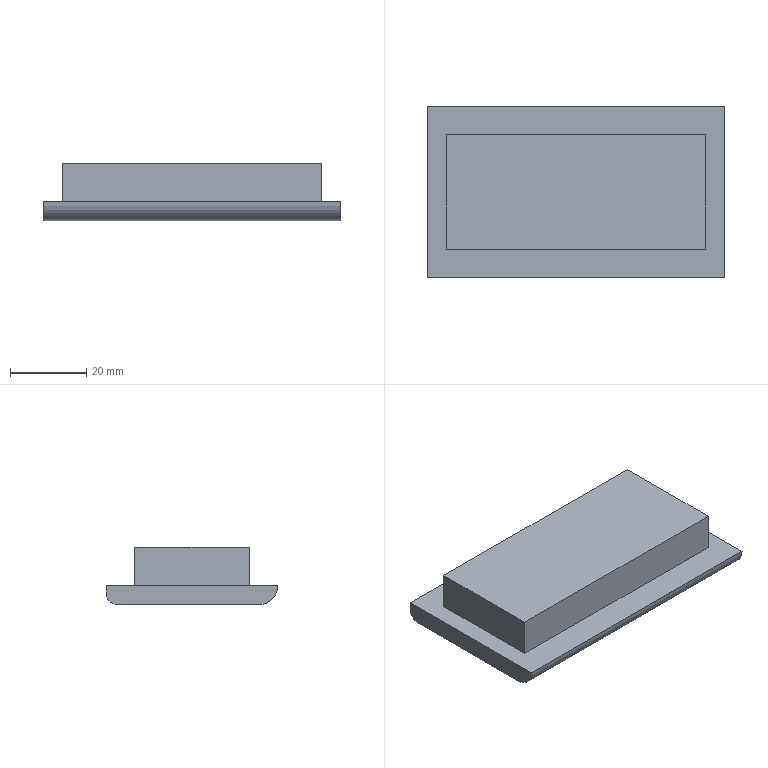Part | SolidWorks | features Fillet 3, ICE 2, Extrusion 1 | 1 solid | 18 faces | box 78 x 45 x 15 mm | volume 24133 mm3 | plane 15 | cylinder 3 | commonest cylinder face diameters 10 x2 6 x1
STEP:
#1=CARTESIAN_POINT('',(-39.,22.5,5.));
#2=VERTEX_POINT('',#1);
#3=CARTESIAN_POINT('',(-39.,-22.5,5.));
#4=VERTEX_POINT('',#3);
#5=CARTESIAN_POINT('',(-39.,-22.5,5.));
#6=DIRECTION('',(0.,-1.,0.));
#7=VECTOR('',#6,1000.);
#8=LINE('',#5,#7);
#9=EDGE_CURVE('',#2,#4,#8,.T.);
#10=ORIENTED_EDGE('',*,*,#9,.T.);
#11=CARTESIAN_POINT('',(39.,-22.5,5.));
#12=VERTEX_POINT('',#11);
#13=CARTESIAN_POINT('',(39.,-22.5,5.));
#14=DIRECTION('',(1.,0.,0.));
#15=VECTOR('',#14,1000.);
#16=LINE('',#13,#15);
#17=EDGE_CURVE('',#4,#12,#16,.T.);
#18=ORIENTED_EDGE('',*,*,#17,.T.);
#19=CARTESIAN_POINT('',(39.,22.5,5.));
#20=VERTEX_POINT('',#19);
#21=CARTESIAN_POINT('',(39.,-22.5,5.));
#22=DIRECTION('',(0.,1.,0.));
#23=VECTOR('',#22,1000.);
#24=LINE('',#21,#23);
#25=EDGE_CURVE('',#12,#20,#24,.T.);
#26=ORIENTED_EDGE('',*,*,#25,.T.);
#27=CARTESIAN_POINT('',(39.,22.5,5.));
#28=DIRECTION('',(-1.,0.,0.));
#29=VECTOR('',#28,1000.);
#30=LINE('',#27,#29);
#31=EDGE_CURVE('',#20,#2,#30,.T.);
#32=ORIENTED_EDGE('',*,*,#31,.T.);
#33=EDGE_LOOP('',(#10,#18,#26,#32));
#34=FACE_OUTER_BOUND('',#33,.T.);
#35=CARTESIAN_POINT('',(-34.,-15.,5.));
#36=VERTEX_POINT('',#35);
#37=CARTESIAN_POINT('',(34.,-15.,5.));
#38=VERTEX_POINT('',#37);
#39=CARTESIAN_POINT('',(34.,-15.,5.));
#40=DIRECTION('',(1.,0.,0.));
#41=VECTOR('',#40,1000.);
#42=LINE('',#39,#41);
#43=EDGE_CURVE('',#36,#38,#42,.T.);
#44=ORIENTED_EDGE('',*,*,#43,.F.);
#45=CARTESIAN_POINT('',(-34.,15.,5.));
#46=VERTEX_POINT('',#45);
#47=CARTESIAN_POINT('',(-34.,-15.,5.));
#48=DIRECTION('',(0.,-1.,0.));
#49=VECTOR('',#48,1000.);
#50=LINE('',#47,#49);
#51=EDGE_CURVE('',#46,#36,#50,.T.);
#52=ORIENTED_EDGE('',*,*,#51,.F.);
#53=CARTESIAN_POINT('',(34.,15.,5.));
#54=VERTEX_POINT('',#53);
#55=CARTESIAN_POINT('',(34.,15.,5.));
#56=DIRECTION('',(-1.,0.,0.));
#57=VECTOR('',#56,1000.);
#58=LINE('',#55,#57);
#59=EDGE_CURVE('',#54,#46,#58,.T.);
#60=ORIENTED_EDGE('',*,*,#59,.F.);
#61=CARTESIAN_POINT('',(34.,-15.,5.));
#62=DIRECTION('',(0.,1.,0.));
#63=VECTOR('',#62,1000.);
#64=LINE('',#61,#63);
#65=EDGE_CURVE('',#38,#54,#64,.T.);
#66=ORIENTED_EDGE('',*,*,#65,.F.);
#67=EDGE_LOOP('',(#44,#52,#60,#66));
#68=FACE_BOUND('',#67,.T.);
#69=CARTESIAN_POINT('',(-39.,22.5,5.));
#70=DIRECTION('',(0.,0.,1.));
#71=DIRECTION('',(1.,0.,0.));
#72=AXIS2_PLACEMENT_3D('',#69,#70,#71);
#73=PLANE('',#72);
#74=ADVANCED_FACE('',(#34,#68),#73,.T.);
#75=CARTESIAN_POINT('',(-39.,19.5,0.));
#76=VERTEX_POINT('',#75);
#77=CARTESIAN_POINT('',(-39.,-17.5,0.));
#78=VERTEX_POINT('',#77);
#79=CARTESIAN_POINT('',(-39.,-22.5,0.));
#80=DIRECTION('',(0.,-1.,0.));
#81=VECTOR('',#80,1000.);
#82=LINE('',#79,#81);
#83=EDGE_CURVE('',#76,#78,#82,.T.);
#84=ORIENTED_EDGE('',*,*,#83,.T.);
#85=CARTESIAN_POINT('',(-39.,-17.5,5.));
#86=DIRECTION('',(-1.,0.,0.));
#87=DIRECTION('',(0.,0.,-1.));
#88=AXIS2_PLACEMENT_3D('',#85,#86,#87);
#89=CIRCLE('',#88,5.);
#90=EDGE_CURVE('',#78,#4,#89,.T.);
#91=ORIENTED_EDGE('',*,*,#90,.T.);
#92=ORIENTED_EDGE('',*,*,#9,.F.);
#93=CARTESIAN_POINT('',(-39.,22.5,3.));
#94=VERTEX_POINT('',#93);
#95=CARTESIAN_POINT('',(-39.,22.5,5.));
#96=DIRECTION('',(0.,0.,-1.));
#97=VECTOR('',#96,1000.);
#98=LINE('',#95,#97);
#99=EDGE_CURVE('',#2,#94,#98,.T.);
#100=ORIENTED_EDGE('',*,*,#99,.T.);
#101=CARTESIAN_POINT('',(-39.,19.5,3.));
#102=DIRECTION('',(-1.,0.,0.));
#103=DIRECTION('',(0.,0.,-1.));
#104=AXIS2_PLACEMENT_3D('',#101,#102,#103);
#105=CIRCLE('',#104,3.);
#106=EDGE_CURVE('',#94,#76,#105,.T.);
#107=ORIENTED_EDGE('',*,*,#106,.T.);
#108=EDGE_LOOP('',(#84,#91,#92,#100,#107));
#109=FACE_OUTER_BOUND('',#108,.T.);
#110=CARTESIAN_POINT('',(-39.,-22.5,5.));
#111=DIRECTION('',(1.,0.,0.));
#112=DIRECTION('',(0.,0.,-1.));
#113=AXIS2_PLACEMENT_3D('',#110,#111,#112);
#114=PLANE('',#113);
#115=ADVANCED_FACE('',(#109),#114,.F.);
#116=ORIENTED_EDGE('',*,*,#25,.F.);
#117=CARTESIAN_POINT('',(39.,-17.5,0.));
#118=VERTEX_POINT('',#117);
#119=CARTESIAN_POINT('',(39.,-17.5,5.));
#120=DIRECTION('',(1.,0.,0.));
#121=DIRECTION('',(0.,0.,1.));
#122=AXIS2_PLACEMENT_3D('',#119,#120,#121);
#123=CIRCLE('',#122,5.);
#124=EDGE_CURVE('',#12,#118,#123,.T.);
#125=ORIENTED_EDGE('',*,*,#124,.T.);
#126=CARTESIAN_POINT('',(39.,19.5,0.));
#127=VERTEX_POINT('',#126);
#128=CARTESIAN_POINT('',(39.,-22.5,0.));
#129=DIRECTION('',(0.,1.,0.));
#130=VECTOR('',#129,1000.);
#131=LINE('',#128,#130);
#132=EDGE_CURVE('',#118,#127,#131,.T.);
#133=ORIENTED_EDGE('',*,*,#132,.T.);
#134=CARTESIAN_POINT('',(39.,22.5,3.));
#135=VERTEX_POINT('',#134);
#136=CARTESIAN_POINT('',(39.,19.5,3.));
#137=DIRECTION('',(1.,0.,0.));
#138=DIRECTION('',(0.,0.,1.));
#139=AXIS2_PLACEMENT_3D('',#136,#137,#138);
#140=CIRCLE('',#139,3.);
#141=EDGE_CURVE('',#127,#135,#140,.T.);
#142=ORIENTED_EDGE('',*,*,#141,.T.);
#143=CARTESIAN_POINT('',(39.,22.5,5.));
#144=DIRECTION('',(0.,0.,-1.));
#145=VECTOR('',#144,1000.);
#146=LINE('',#143,#145);
#147=EDGE_CURVE('',#20,#135,#146,.T.);
#148=ORIENTED_EDGE('',*,*,#147,.F.);
#149=EDGE_LOOP('',(#116,#125,#133,#142,#148));
#150=FACE_OUTER_BOUND('',#149,.T.);
#151=CARTESIAN_POINT('',(39.,-22.5,5.));
#152=DIRECTION('',(-1.,0.,0.));
#153=DIRECTION('',(0.,0.,1.));
#154=AXIS2_PLACEMENT_3D('',#151,#152,#153);
#155=PLANE('',#154);
#156=ADVANCED_FACE('',(#150),#155,.F.);
#157=ORIENTED_EDGE('',*,*,#147,.T.);
#158=CARTESIAN_POINT('',(39.,22.5,3.));
#159=DIRECTION('',(-1.,0.,0.));
#160=VECTOR('',#159,1000.);
#161=LINE('',#158,#160);
#162=EDGE_CURVE('',#135,#94,#161,.T.);
#163=ORIENTED_EDGE('',*,*,#162,.T.);
#164=ORIENTED_EDGE('',*,*,#99,.F.);
#165=ORIENTED_EDGE('',*,*,#31,.F.);
#166=EDGE_LOOP('',(#157,#163,#164,#165));
#167=FACE_OUTER_BOUND('',#166,.T.);
#168=CARTESIAN_POINT('',(39.,22.5,5.));
#169=DIRECTION('',(0.,-1.,0.));
#170=DIRECTION('',(1.,0.,0.));
#171=AXIS2_PLACEMENT_3D('',#168,#169,#170);
#172=PLANE('',#171);
#173=ADVANCED_FACE('',(#167),#172,.F.);
#174=CARTESIAN_POINT('',(29.243,-11.594,0.));
#175=VERTEX_POINT('',#174);
#176=CARTESIAN_POINT('',(-29.243,-11.594,0.));
#177=VERTEX_POINT('',#176);
#178=CARTESIAN_POINT('',(-29.243,-11.594,0.));
#179=DIRECTION('',(-1.,0.,0.));
#180=VECTOR('',#179,1000.);
#181=LINE('',#178,#180);
#182=EDGE_CURVE('',#175,#177,#181,.T.);
#183=ORIENTED_EDGE('',*,*,#182,.F.);
#184=CARTESIAN_POINT('',(29.243,11.594,0.));
#185=VERTEX_POINT('',#184);
#186=CARTESIAN_POINT('',(29.243,-11.594,0.));
#187=DIRECTION('',(0.,-1.,0.));
#188=VECTOR('',#187,1000.);
#189=LINE('',#186,#188);
#190=EDGE_CURVE('',#185,#175,#189,.T.);
#191=ORIENTED_EDGE('',*,*,#190,.F.);
#192=CARTESIAN_POINT('',(-29.243,11.594,0.));
#193=VERTEX_POINT('',#192);
#194=CARTESIAN_POINT('',(-29.243,11.594,0.));
#195=DIRECTION('',(1.,0.,0.));
#196=VECTOR('',#195,1000.);
#197=LINE('',#194,#196);
#198=EDGE_CURVE('',#193,#185,#197,.T.);
#199=ORIENTED_EDGE('',*,*,#198,.F.);
#200=CARTESIAN_POINT('',(-29.243,-11.594,0.));
#201=DIRECTION('',(0.,1.,0.));
#202=VECTOR('',#201,1000.);
#203=LINE('',#200,#202);
#204=EDGE_CURVE('',#177,#193,#203,.T.);
#205=ORIENTED_EDGE('',*,*,#204,.F.);
#206=EDGE_LOOP('',(#183,#191,#199,#205));
#207=FACE_BOUND('',#206,.T.);
#208=ORIENTED_EDGE('',*,*,#132,.F.);
#209=CARTESIAN_POINT('',(-39.,-17.5,0.));
#210=DIRECTION('',(-1.,0.,0.));
#211=VECTOR('',#210,1000.);
#212=LINE('',#209,#211);
#213=EDGE_CURVE('',#118,#78,#212,.T.);
#214=ORIENTED_EDGE('',*,*,#213,.T.);
#215=ORIENTED_EDGE('',*,*,#83,.F.);
#216=CARTESIAN_POINT('',(-39.,19.5,0.));
#217=DIRECTION('',(1.,0.,0.));
#218=VECTOR('',#217,1000.);
#219=LINE('',#216,#218);
#220=EDGE_CURVE('',#76,#127,#219,.T.);
#221=ORIENTED_EDGE('',*,*,#220,.T.);
#222=EDGE_LOOP('',(#208,#214,#215,#221));
#223=FACE_OUTER_BOUND('',#222,.T.);
#224=CARTESIAN_POINT('',(-39.,22.5,0.));
#225=DIRECTION('',(0.,0.,1.));
#226=DIRECTION('',(1.,0.,0.));
#227=AXIS2_PLACEMENT_3D('',#224,#225,#226);
#228=PLANE('',#227);
#229=ADVANCED_FACE('',(#207,#223),#228,.F.);
#230=ORIENTED_EDGE('',*,*,#51,.T.);
#231=CARTESIAN_POINT('',(-34.,-15.,15.));
#232=VERTEX_POINT('',#231);
#233=CARTESIAN_POINT('',(-34.,-15.,15.));
#234=DIRECTION('',(0.,0.,-1.));
#235=VECTOR('',#234,1000.);
#236=LINE('',#233,#235);
#237=EDGE_CURVE('',#232,#36,#236,.T.);
#238=ORIENTED_EDGE('',*,*,#237,.F.);
#239=CARTESIAN_POINT('',(-34.,15.,15.));
#240=VERTEX_POINT('',#239);
#241=CARTESIAN_POINT('',(-34.,-15.,15.));
#242=DIRECTION('',(0.,-1.,0.));
#243=VECTOR('',#242,1000.);
#244=LINE('',#241,#243);
#245=EDGE_CURVE('',#240,#232,#244,.T.);
#246=ORIENTED_EDGE('',*,*,#245,.F.);
#247=CARTESIAN_POINT('',(-34.,15.,15.));
#248=DIRECTION('',(0.,0.,-1.));
#249=VECTOR('',#248,1000.);
#250=LINE('',#247,#249);
#251=EDGE_CURVE('',#240,#46,#250,.T.);
#252=ORIENTED_EDGE('',*,*,#251,.T.);
#253=EDGE_LOOP('',(#230,#238,#246,#252));
#254=FACE_OUTER_BOUND('',#253,.T.);
#255=CARTESIAN_POINT('',(-34.,-15.,15.));
#256=DIRECTION('',(1.,0.,0.));
#257=DIRECTION('',(0.,0.,-1.));
#258=AXIS2_PLACEMENT_3D('',#255,#256,#257);
#259=PLANE('',#258);
#260=ADVANCED_FACE('',(#254),#259,.F.);
#261=ORIENTED_EDGE('',*,*,#43,.T.);
#262=CARTESIAN_POINT('',(34.,-15.,15.));
#263=VERTEX_POINT('',#262);
#264=CARTESIAN_POINT('',(34.,-15.,15.));
#265=DIRECTION('',(0.,0.,-1.));
#266=VECTOR('',#265,1000.);
#267=LINE('',#264,#266);
#268=EDGE_CURVE('',#263,#38,#267,.T.);
#269=ORIENTED_EDGE('',*,*,#268,.F.);
#270=CARTESIAN_POINT('',(34.,-15.,15.));
#271=DIRECTION('',(1.,0.,0.));
#272=VECTOR('',#271,1000.);
#273=LINE('',#270,#272);
#274=EDGE_CURVE('',#232,#263,#273,.T.);
#275=ORIENTED_EDGE('',*,*,#274,.F.);
#276=ORIENTED_EDGE('',*,*,#237,.T.);
#277=EDGE_LOOP('',(#261,#269,#275,#276));
#278=FACE_OUTER_BOUND('',#277,.T.);
#279=CARTESIAN_POINT('',(34.,-15.,15.));
#280=DIRECTION('',(0.,1.,0.));
#281=DIRECTION('',(-1.,0.,0.));
#282=AXIS2_PLACEMENT_3D('',#279,#280,#281);
#283=PLANE('',#282);
#284=ADVANCED_FACE('',(#278),#283,.F.);
#285=ORIENTED_EDGE('',*,*,#65,.T.);
#286=CARTESIAN_POINT('',(34.,15.,15.));
#287=VERTEX_POINT('',#286);
#288=CARTESIAN_POINT('',(34.,15.,15.));
#289=DIRECTION('',(0.,0.,-1.));
#290=VECTOR('',#289,1000.);
#291=LINE('',#288,#290);
#292=EDGE_CURVE('',#287,#54,#291,.T.);
#293=ORIENTED_EDGE('',*,*,#292,.F.);
#294=CARTESIAN_POINT('',(34.,-15.,15.));
#295=DIRECTION('',(0.,1.,0.));
#296=VECTOR('',#295,1000.);
#297=LINE('',#294,#296);
#298=EDGE_CURVE('',#263,#287,#297,.T.);
#299=ORIENTED_EDGE('',*,*,#298,.F.);
#300=ORIENTED_EDGE('',*,*,#268,.T.);
#301=EDGE_LOOP('',(#285,#293,#299,#300));
#302=FACE_OUTER_BOUND('',#301,.T.);
#303=CARTESIAN_POINT('',(34.,-15.,15.));
#304=DIRECTION('',(-1.,0.,0.));
#305=DIRECTION('',(0.,0.,1.));
#306=AXIS2_PLACEMENT_3D('',#303,#304,#305);
#307=PLANE('',#306);
#308=ADVANCED_FACE('',(#302),#307,.F.);
#309=ORIENTED_EDGE('',*,*,#59,.T.);
#310=ORIENTED_EDGE('',*,*,#251,.F.);
#311=CARTESIAN_POINT('',(34.,15.,15.));
#312=DIRECTION('',(-1.,0.,0.));
#313=VECTOR('',#312,1000.);
#314=LINE('',#311,#313);
#315=EDGE_CURVE('',#287,#240,#314,.T.);
#316=ORIENTED_EDGE('',*,*,#315,.F.);
#317=ORIENTED_EDGE('',*,*,#292,.T.);
#318=EDGE_LOOP('',(#309,#310,#316,#317));
#319=FACE_OUTER_BOUND('',#318,.T.);
#320=CARTESIAN_POINT('',(34.,15.,15.));
#321=DIRECTION('',(0.,-1.,0.));
#322=DIRECTION('',(1.,0.,0.));
#323=AXIS2_PLACEMENT_3D('',#320,#321,#322);
#324=PLANE('',#323);
#325=ADVANCED_FACE('',(#319),#324,.F.);
#326=ORIENTED_EDGE('',*,*,#245,.T.);
#327=ORIENTED_EDGE('',*,*,#274,.T.);
#328=ORIENTED_EDGE('',*,*,#298,.T.);
#329=ORIENTED_EDGE('',*,*,#315,.T.);
#330=EDGE_LOOP('',(#326,#327,#328,#329));
#331=FACE_OUTER_BOUND('',#330,.T.);
#332=CARTESIAN_POINT('',(-34.,15.,15.));
#333=DIRECTION('',(0.,0.,1.));
#334=DIRECTION('',(1.,0.,0.));
#335=AXIS2_PLACEMENT_3D('',#332,#333,#334);
#336=PLANE('',#335);
#337=ADVANCED_FACE('',(#331),#336,.T.);
#338=ORIENTED_EDGE('',*,*,#141,.F.);
#339=ORIENTED_EDGE('',*,*,#220,.F.);
#340=ORIENTED_EDGE('',*,*,#106,.F.);
#341=ORIENTED_EDGE('',*,*,#162,.F.);
#342=EDGE_LOOP('',(#338,#339,#340,#341));
#343=FACE_OUTER_BOUND('',#342,.T.);
#344=CARTESIAN_POINT('',(39.,19.5,3.));
#345=DIRECTION('',(-1.,0.,0.));
#346=DIRECTION('',(0.,-1.,0.));
#347=AXIS2_PLACEMENT_3D('',#344,#345,#346);
#348=CYLINDRICAL_SURFACE('',#347,3.);
#349=ADVANCED_FACE('',(#343),#348,.T.);
#350=ORIENTED_EDGE('',*,*,#90,.F.);
#351=ORIENTED_EDGE('',*,*,#213,.F.);
#352=ORIENTED_EDGE('',*,*,#124,.F.);
#353=ORIENTED_EDGE('',*,*,#17,.F.);
#354=EDGE_LOOP('',(#350,#351,#352,#353));
#355=FACE_OUTER_BOUND('',#354,.T.);
#356=CARTESIAN_POINT('',(39.,-17.5,5.));
#357=DIRECTION('',(1.,0.,0.));
#358=DIRECTION('',(0.,1.,0.));
#359=AXIS2_PLACEMENT_3D('',#356,#357,#358);
#360=CYLINDRICAL_SURFACE('',#359,5.);
#361=ADVANCED_FACE('',(#355),#360,.T.);
#362=CARTESIAN_POINT('',(29.243,-11.594,5.));
#363=VERTEX_POINT('',#362);
#364=CARTESIAN_POINT('',(29.243,-11.594,10.));
#365=DIRECTION('',(0.,0.,-1.));
#366=VECTOR('',#365,1000.);
#367=LINE('',#364,#366);
#368=EDGE_CURVE('',#363,#175,#367,.T.);
#369=ORIENTED_EDGE('',*,*,#368,.F.);
#370=CARTESIAN_POINT('',(29.243,-6.594,10.));
#371=VERTEX_POINT('',#370);
#372=CARTESIAN_POINT('',(29.243,-6.594,5.));
#373=DIRECTION('',(-1.,0.,0.));
#374=DIRECTION('',(0.,0.,-1.));
#375=AXIS2_PLACEMENT_3D('',#372,#373,#374);
#376=CIRCLE('',#375,5.);
#377=EDGE_CURVE('',#363,#371,#376,.T.);
#378=ORIENTED_EDGE('',*,*,#377,.T.);
#379=CARTESIAN_POINT('',(29.243,11.594,10.));
#380=VERTEX_POINT('',#379);
#381=CARTESIAN_POINT('',(29.243,-11.594,10.));
#382=DIRECTION('',(0.,-1.,0.));
#383=VECTOR('',#382,1000.);
#384=LINE('',#381,#383);
#385=EDGE_CURVE('',#380,#371,#384,.T.);
#386=ORIENTED_EDGE('',*,*,#385,.F.);
#387=CARTESIAN_POINT('',(29.243,11.594,10.));
#388=DIRECTION('',(0.,0.,-1.));
#389=VECTOR('',#388,1000.);
#390=LINE('',#387,#389);
#391=EDGE_CURVE('',#380,#185,#390,.T.);
#392=ORIENTED_EDGE('',*,*,#391,.T.);
#393=ORIENTED_EDGE('',*,*,#190,.T.);
#394=EDGE_LOOP('',(#369,#378,#386,#392,#393));
#395=FACE_OUTER_BOUND('',#394,.T.);
#396=CARTESIAN_POINT('',(29.243,-11.594,10.));
#397=DIRECTION('',(1.,0.,0.));
#398=DIRECTION('',(0.,0.,-1.));
#399=AXIS2_PLACEMENT_3D('',#396,#397,#398);
#400=PLANE('',#399);
#401=ADVANCED_FACE('',(#395),#400,.F.);
#402=ORIENTED_EDGE('',*,*,#198,.T.);
#403=ORIENTED_EDGE('',*,*,#391,.F.);
#404=CARTESIAN_POINT('',(-29.243,11.594,10.));
#405=VERTEX_POINT('',#404);
#406=CARTESIAN_POINT('',(-29.243,11.594,10.));
#407=DIRECTION('',(1.,0.,0.));
#408=VECTOR('',#407,1000.);
#409=LINE('',#406,#408);
#410=EDGE_CURVE('',#405,#380,#409,.T.);
#411=ORIENTED_EDGE('',*,*,#410,.F.);
#412=CARTESIAN_POINT('',(-29.243,11.594,10.));
#413=DIRECTION('',(0.,0.,-1.));
#414=VECTOR('',#413,1000.);
#415=LINE('',#412,#414);
#416=EDGE_CURVE('',#405,#193,#415,.T.);
#417=ORIENTED_EDGE('',*,*,#416,.T.);
#418=EDGE_LOOP('',(#402,#403,#411,#417));
#419=FACE_OUTER_BOUND('',#418,.T.);
#420=CARTESIAN_POINT('',(-29.243,11.594,10.));
#421=DIRECTION('',(0.,1.,0.));
#422=DIRECTION('',(0.,0.,1.));
#423=AXIS2_PLACEMENT_3D('',#420,#421,#422);
#424=PLANE('',#423);
#425=ADVANCED_FACE('',(#419),#424,.F.);
#426=CARTESIAN_POINT('',(-29.243,-6.594,10.));
#427=VERTEX_POINT('',#426);
#428=CARTESIAN_POINT('',(-29.243,-11.594,10.));
#429=DIRECTION('',(0.,1.,0.));
#430=VECTOR('',#429,1000.);
#431=LINE('',#428,#430);
#432=EDGE_CURVE('',#427,#405,#431,.T.);
#433=ORIENTED_EDGE('',*,*,#432,.F.);
#434=CARTESIAN_POINT('',(-29.243,-11.594,5.));
#435=VERTEX_POINT('',#434);
#436=CARTESIAN_POINT('',(-29.243,-6.594,5.));
#437=DIRECTION('',(1.,0.,0.));
#438=DIRECTION('',(0.,0.,1.));
#439=AXIS2_PLACEMENT_3D('',#436,#437,#438);
#440=CIRCLE('',#439,5.);
#441=EDGE_CURVE('',#427,#435,#440,.T.);
#442=ORIENTED_EDGE('',*,*,#441,.T.);
#443=CARTESIAN_POINT('',(-29.243,-11.594,10.));
#444=DIRECTION('',(0.,0.,-1.));
#445=VECTOR('',#444,1000.);
#446=LINE('',#443,#445);
#447=EDGE_CURVE('',#435,#177,#446,.T.);
#448=ORIENTED_EDGE('',*,*,#447,.T.);
#449=ORIENTED_EDGE('',*,*,#204,.T.);
#450=ORIENTED_EDGE('',*,*,#416,.F.);
#451=EDGE_LOOP('',(#433,#442,#448,#449,#450));
#452=FACE_OUTER_BOUND('',#451,.T.);
#453=CARTESIAN_POINT('',(-29.243,-11.594,10.));
#454=DIRECTION('',(-1.,0.,0.));
#455=DIRECTION('',(0.,0.,1.));
#456=AXIS2_PLACEMENT_3D('',#453,#454,#455);
#457=PLANE('',#456);
#458=ADVANCED_FACE('',(#452),#457,.F.);
#459=ORIENTED_EDGE('',*,*,#447,.F.);
#460=CARTESIAN_POINT('',(-29.243,-11.594,5.));
#461=DIRECTION('',(1.,0.,0.));
#462=VECTOR('',#461,1000.);
#463=LINE('',#460,#462);
#464=EDGE_CURVE('',#435,#363,#463,.T.);
#465=ORIENTED_EDGE('',*,*,#464,.T.);
#466=ORIENTED_EDGE('',*,*,#368,.T.);
#467=ORIENTED_EDGE('',*,*,#182,.T.);
#468=EDGE_LOOP('',(#459,#465,#466,#467));
#469=FACE_OUTER_BOUND('',#468,.T.);
#470=CARTESIAN_POINT('',(-29.243,-11.594,10.));
#471=DIRECTION('',(0.,-1.,0.));
#472=DIRECTION('',(0.,0.,-1.));
#473=AXIS2_PLACEMENT_3D('',#470,#471,#472);
#474=PLANE('',#473);
#475=ADVANCED_FACE('',(#469),#474,.F.);
#476=ORIENTED_EDGE('',*,*,#385,.T.);
#477=CARTESIAN_POINT('',(29.243,-6.594,10.));
#478=DIRECTION('',(-1.,0.,0.));
#479=VECTOR('',#478,1000.);
#480=LINE('',#477,#479);
#481=EDGE_CURVE('',#371,#427,#480,.T.);
#482=ORIENTED_EDGE('',*,*,#481,.T.);
#483=ORIENTED_EDGE('',*,*,#432,.T.);
#484=ORIENTED_EDGE('',*,*,#410,.T.);
#485=EDGE_LOOP('',(#476,#482,#483,#484));
#486=FACE_OUTER_BOUND('',#485,.T.);
#487=CARTESIAN_POINT('',(29.243,11.594,10.));
#488=DIRECTION('',(0.,0.,-1.));
#489=DIRECTION('',(-1.,0.,0.));
#490=AXIS2_PLACEMENT_3D('',#487,#488,#489);
#491=PLANE('',#490);
#492=ADVANCED_FACE('',(#486),#491,.T.);
#493=ORIENTED_EDGE('',*,*,#377,.F.);
#494=ORIENTED_EDGE('',*,*,#464,.F.);
#495=ORIENTED_EDGE('',*,*,#441,.F.);
#496=ORIENTED_EDGE('',*,*,#481,.F.);
#497=EDGE_LOOP('',(#493,#494,#495,#496));
#498=FACE_OUTER_BOUND('',#497,.T.);
#499=CARTESIAN_POINT('',(29.243,-6.594,5.));
#500=DIRECTION('',(-1.,0.,0.));
#501=DIRECTION('',(0.,0.,1.));
#502=AXIS2_PLACEMENT_3D('',#499,#500,#501);
#503=CYLINDRICAL_SURFACE('',#502,5.);
#504=ADVANCED_FACE('',(#498),#503,.F.);
#505=CLOSED_SHELL('',(#74,#115,#156,#173,#229,#260,#284,#308,#325,#337,#349,#361,#401,#425,#458,#475,#492,#504));
#506=MANIFOLD_SOLID_BREP('',#505);
#507=CARTESIAN_POINT('',(0.,0.,0.));
#508=DIRECTION('',(0.,0.,1.));
#509=DIRECTION('',(1.,0.,0.));
#510=AXIS2_PLACEMENT_3D('',#507,#508,#509);
#511=(LENGTH_UNIT()NAMED_UNIT(*)SI_UNIT(.MILLI.,.METRE.));
#512=UNCERTAINTY_MEASURE_WITH_UNIT(LENGTH_MEASURE(0.00001),#511,'','');
#513=(NAMED_UNIT(*)PLANE_ANGLE_UNIT()SI_UNIT($,.RADIAN.));
#514=(NAMED_UNIT(*)SI_UNIT($,.STERADIAN.)SOLID_ANGLE_UNIT());
#515=(GEOMETRIC_REPRESENTATION_CONTEXT(3)GLOBAL_UNCERTAINTY_ASSIGNED_CONTEXT((#512))GLOBAL_UNIT_ASSIGNED_CONTEXT((#511,#513,#514))REPRESENTATION_CONTEXT('',''));
#516=ADVANCED_BREP_SHAPE_REPRESENTATION('',(#506,#510),#515);